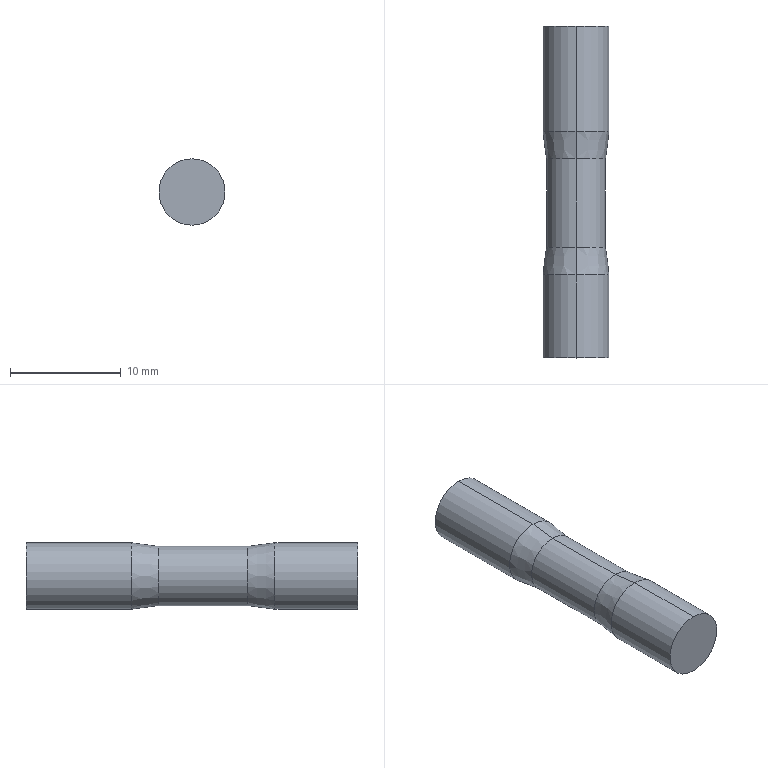Part | SolidWorks | features Revolution 1 | 1 solid | 12 faces | box 6 x 30 x 6 mm | volume 787.114 mm3 | cylinder 6 | cone 4 | plane 2 | commonest cylinder face diameters 6 x4 5.35 x2
STEP:
#1=CARTESIAN_POINT('',(0.,-22.5,-3.));
#2=VERTEX_POINT('',#1);
#3=CARTESIAN_POINT('',(0.,-22.5,3.));
#4=VERTEX_POINT('',#3);
#5=CARTESIAN_POINT('',(0.,-22.5,0.));
#6=DIRECTION('',(0.,-1.,0.));
#7=DIRECTION('',(0.,0.,-1.));
#8=AXIS2_PLACEMENT_3D('',#5,#6,#7);
#9=CIRCLE('',#8,3.);
#10=EDGE_CURVE('',#2,#4,#9,.T.);
#11=ORIENTED_EDGE('',*,*,#10,.T.);
#12=CARTESIAN_POINT('',(0.,-30.,3.));
#13=VERTEX_POINT('',#12);
#14=CARTESIAN_POINT('',(0.,-30.,3.));
#15=DIRECTION('',(0.,-1.,0.));
#16=VECTOR('',#15,1000.);
#17=LINE('',#14,#16);
#18=EDGE_CURVE('',#4,#13,#17,.T.);
#19=ORIENTED_EDGE('',*,*,#18,.T.);
#20=CARTESIAN_POINT('',(0.,-30.,-3.));
#21=VERTEX_POINT('',#20);
#22=CARTESIAN_POINT('',(0.,-30.,0.));
#23=DIRECTION('',(0.,-1.,0.));
#24=DIRECTION('',(0.,0.,-1.));
#25=AXIS2_PLACEMENT_3D('',#22,#23,#24);
#26=CIRCLE('',#25,3.);
#27=EDGE_CURVE('',#21,#13,#26,.T.);
#28=ORIENTED_EDGE('',*,*,#27,.F.);
#29=CARTESIAN_POINT('',(0.,-30.,-3.));
#30=DIRECTION('',(0.,-1.,0.));
#31=VECTOR('',#30,1000.);
#32=LINE('',#29,#31);
#33=EDGE_CURVE('',#2,#21,#32,.T.);
#34=ORIENTED_EDGE('',*,*,#33,.F.);
#35=EDGE_LOOP('',(#11,#19,#28,#34));
#36=FACE_OUTER_BOUND('',#35,.T.);
#37=CARTESIAN_POINT('',(0.,-30.,0.));
#38=DIRECTION('',(0.,-1.,0.));
#39=DIRECTION('',(0.,0.,-1.));
#40=AXIS2_PLACEMENT_3D('',#37,#38,#39);
#41=CYLINDRICAL_SURFACE('',#40,3.);
#42=ADVANCED_FACE('',(#36),#41,.T.);
#43=CARTESIAN_POINT('',(0.,-20.,-2.675));
#44=VERTEX_POINT('',#43);
#45=CARTESIAN_POINT('',(0.,-20.,2.675));
#46=VERTEX_POINT('',#45);
#47=CARTESIAN_POINT('',(0.,-20.,0.));
#48=DIRECTION('',(0.,-1.,0.));
#49=DIRECTION('',(0.,0.,-1.));
#50=AXIS2_PLACEMENT_3D('',#47,#48,#49);
#51=CIRCLE('',#50,2.675);
#52=EDGE_CURVE('',#44,#46,#51,.T.);
#53=ORIENTED_EDGE('',*,*,#52,.T.);
#54=CARTESIAN_POINT('',(0.,-20.,2.675));
#55=DIRECTION('',(0.,-0.9917,0.1289));
#56=VECTOR('',#55,1000.);
#57=LINE('',#54,#56);
#58=EDGE_CURVE('',#46,#4,#57,.T.);
#59=ORIENTED_EDGE('',*,*,#58,.T.);
#60=ORIENTED_EDGE('',*,*,#10,.F.);
#61=CARTESIAN_POINT('',(0.,-20.,-2.675));
#62=DIRECTION('',(0.,-0.9917,-0.1289));
#63=VECTOR('',#62,1000.);
#64=LINE('',#61,#63);
#65=EDGE_CURVE('',#44,#2,#64,.T.);
#66=ORIENTED_EDGE('',*,*,#65,.F.);
#67=EDGE_LOOP('',(#53,#59,#60,#66));
#68=FACE_OUTER_BOUND('',#67,.T.);
#69=CARTESIAN_POINT('',(0.,-20.,0.));
#70=DIRECTION('',(0.,-1.,0.));
#71=DIRECTION('',(0.,0.,-1.));
#72=AXIS2_PLACEMENT_3D('',#69,#70,#71);
#73=CONICAL_SURFACE('',#72,2.675,0.1293);
#74=ADVANCED_FACE('',(#68),#73,.T.);
#75=CARTESIAN_POINT('',(0.,-12.,-2.675));
#76=VERTEX_POINT('',#75);
#77=CARTESIAN_POINT('',(0.,-12.,2.675));
#78=VERTEX_POINT('',#77);
#79=CARTESIAN_POINT('',(0.,-12.,0.));
#80=DIRECTION('',(0.,-1.,0.));
#81=DIRECTION('',(0.,0.,-1.));
#82=AXIS2_PLACEMENT_3D('',#79,#80,#81);
#83=CIRCLE('',#82,2.675);
#84=EDGE_CURVE('',#76,#78,#83,.T.);
#85=ORIENTED_EDGE('',*,*,#84,.T.);
#86=CARTESIAN_POINT('',(0.,-30.,2.675));
#87=DIRECTION('',(0.,-1.,0.));
#88=VECTOR('',#87,1000.);
#89=LINE('',#86,#88);
#90=EDGE_CURVE('',#78,#46,#89,.T.);
#91=ORIENTED_EDGE('',*,*,#90,.T.);
#92=ORIENTED_EDGE('',*,*,#52,.F.);
#93=CARTESIAN_POINT('',(0.,-30.,-2.675));
#94=DIRECTION('',(0.,-1.,0.));
#95=VECTOR('',#94,1000.);
#96=LINE('',#93,#95);
#97=EDGE_CURVE('',#76,#44,#96,.T.);
#98=ORIENTED_EDGE('',*,*,#97,.F.);
#99=EDGE_LOOP('',(#85,#91,#92,#98));
#100=FACE_OUTER_BOUND('',#99,.T.);
#101=CARTESIAN_POINT('',(0.,-30.,0.));
#102=DIRECTION('',(0.,-1.,0.));
#103=DIRECTION('',(0.,0.,-1.));
#104=AXIS2_PLACEMENT_3D('',#101,#102,#103);
#105=CYLINDRICAL_SURFACE('',#104,2.675);
#106=ADVANCED_FACE('',(#100),#105,.T.);
#107=ORIENTED_EDGE('',*,*,#84,.F.);
#108=CARTESIAN_POINT('',(0.,-9.5,-3.));
#109=VERTEX_POINT('',#108);
#110=CARTESIAN_POINT('',(0.,-9.5,-3.));
#111=DIRECTION('',(0.,0.9917,-0.1289));
#112=VECTOR('',#111,1000.);
#113=LINE('',#110,#112);
#114=EDGE_CURVE('',#76,#109,#113,.T.);
#115=ORIENTED_EDGE('',*,*,#114,.T.);
#116=CARTESIAN_POINT('',(0.,-9.5,3.));
#117=VERTEX_POINT('',#116);
#118=CARTESIAN_POINT('',(0.,-9.5,0.));
#119=DIRECTION('',(0.,-1.,0.));
#120=DIRECTION('',(0.,0.,-1.));
#121=AXIS2_PLACEMENT_3D('',#118,#119,#120);
#122=CIRCLE('',#121,3.);
#123=EDGE_CURVE('',#109,#117,#122,.T.);
#124=ORIENTED_EDGE('',*,*,#123,.T.);
#125=CARTESIAN_POINT('',(0.,-9.5,3.));
#126=DIRECTION('',(0.,0.9917,0.1289));
#127=VECTOR('',#126,1000.);
#128=LINE('',#125,#127);
#129=EDGE_CURVE('',#78,#117,#128,.T.);
#130=ORIENTED_EDGE('',*,*,#129,.F.);
#131=EDGE_LOOP('',(#107,#115,#124,#130));
#132=FACE_OUTER_BOUND('',#131,.T.);
#133=CARTESIAN_POINT('',(0.,-9.5,0.));
#134=DIRECTION('',(0.,1.,0.));
#135=DIRECTION('',(0.,0.,1.));
#136=AXIS2_PLACEMENT_3D('',#133,#134,#135);
#137=CONICAL_SURFACE('',#136,3.,0.1293);
#138=ADVANCED_FACE('',(#132),#137,.T.);
#139=CARTESIAN_POINT('',(0.,0.,-3.));
#140=VERTEX_POINT('',#139);
#141=CARTESIAN_POINT('',(0.,0.,3.));
#142=VERTEX_POINT('',#141);
#143=CARTESIAN_POINT('',(0.,0.,0.));
#144=DIRECTION('',(0.,-1.,0.));
#145=DIRECTION('',(0.,0.,-1.));
#146=AXIS2_PLACEMENT_3D('',#143,#144,#145);
#147=CIRCLE('',#146,3.);
#148=EDGE_CURVE('',#140,#142,#147,.T.);
#149=ORIENTED_EDGE('',*,*,#148,.T.);
#150=CARTESIAN_POINT('',(0.,-30.,3.));
#151=DIRECTION('',(0.,-1.,0.));
#152=VECTOR('',#151,1000.);
#153=LINE('',#150,#152);
#154=EDGE_CURVE('',#142,#117,#153,.T.);
#155=ORIENTED_EDGE('',*,*,#154,.T.);
#156=ORIENTED_EDGE('',*,*,#123,.F.);
#157=CARTESIAN_POINT('',(0.,-30.,-3.));
#158=DIRECTION('',(0.,-1.,0.));
#159=VECTOR('',#158,1000.);
#160=LINE('',#157,#159);
#161=EDGE_CURVE('',#140,#109,#160,.T.);
#162=ORIENTED_EDGE('',*,*,#161,.F.);
#163=EDGE_LOOP('',(#149,#155,#156,#162));
#164=FACE_OUTER_BOUND('',#163,.T.);
#165=CARTESIAN_POINT('',(0.,-30.,0.));
#166=DIRECTION('',(0.,-1.,0.));
#167=DIRECTION('',(0.,0.,-1.));
#168=AXIS2_PLACEMENT_3D('',#165,#166,#167);
#169=CYLINDRICAL_SURFACE('',#168,3.);
#170=ADVANCED_FACE('',(#164),#169,.T.);
#171=ORIENTED_EDGE('',*,*,#148,.F.);
#172=CARTESIAN_POINT('',(0.,0.,0.));
#173=DIRECTION('',(0.,-1.,0.));
#174=DIRECTION('',(0.,0.,-1.));
#175=AXIS2_PLACEMENT_3D('',#172,#173,#174);
#176=CIRCLE('',#175,3.);
#177=EDGE_CURVE('',#142,#140,#176,.T.);
#178=ORIENTED_EDGE('',*,*,#177,.F.);
#179=EDGE_LOOP('',(#171,#178));
#180=FACE_OUTER_BOUND('',#179,.T.);
#181=CARTESIAN_POINT('',(0.,0.,0.));
#182=DIRECTION('',(0.,-1.,0.));
#183=DIRECTION('',(0.,0.,-1.));
#184=AXIS2_PLACEMENT_3D('',#181,#182,#183);
#185=PLANE('',#184);
#186=ADVANCED_FACE('',(#180),#185,.F.);
#187=ORIENTED_EDGE('',*,*,#154,.F.);
#188=ORIENTED_EDGE('',*,*,#177,.T.);
#189=ORIENTED_EDGE('',*,*,#161,.T.);
#190=CARTESIAN_POINT('',(0.,-9.5,0.));
#191=DIRECTION('',(0.,-1.,0.));
#192=DIRECTION('',(0.,0.,-1.));
#193=AXIS2_PLACEMENT_3D('',#190,#191,#192);
#194=CIRCLE('',#193,3.);
#195=EDGE_CURVE('',#117,#109,#194,.T.);
#196=ORIENTED_EDGE('',*,*,#195,.F.);
#197=EDGE_LOOP('',(#187,#188,#189,#196));
#198=FACE_OUTER_BOUND('',#197,.T.);
#199=CARTESIAN_POINT('',(0.,-30.,0.));
#200=DIRECTION('',(0.,-1.,0.));
#201=DIRECTION('',(0.,0.,-1.));
#202=AXIS2_PLACEMENT_3D('',#199,#200,#201);
#203=CYLINDRICAL_SURFACE('',#202,3.);
#204=ADVANCED_FACE('',(#198),#203,.T.);
#205=ORIENTED_EDGE('',*,*,#114,.F.);
#206=CARTESIAN_POINT('',(0.,-12.,0.));
#207=DIRECTION('',(0.,-1.,0.));
#208=DIRECTION('',(0.,0.,-1.));
#209=AXIS2_PLACEMENT_3D('',#206,#207,#208);
#210=CIRCLE('',#209,2.675);
#211=EDGE_CURVE('',#78,#76,#210,.T.);
#212=ORIENTED_EDGE('',*,*,#211,.F.);
#213=ORIENTED_EDGE('',*,*,#129,.T.);
#214=ORIENTED_EDGE('',*,*,#195,.T.);
#215=EDGE_LOOP('',(#205,#212,#213,#214));
#216=FACE_OUTER_BOUND('',#215,.T.);
#217=CARTESIAN_POINT('',(0.,-9.5,0.));
#218=DIRECTION('',(0.,1.,0.));
#219=DIRECTION('',(0.,0.,1.));
#220=AXIS2_PLACEMENT_3D('',#217,#218,#219);
#221=CONICAL_SURFACE('',#220,3.,0.1293);
#222=ADVANCED_FACE('',(#216),#221,.T.);
#223=ORIENTED_EDGE('',*,*,#90,.F.);
#224=ORIENTED_EDGE('',*,*,#211,.T.);
#225=ORIENTED_EDGE('',*,*,#97,.T.);
#226=CARTESIAN_POINT('',(0.,-20.,0.));
#227=DIRECTION('',(0.,-1.,0.));
#228=DIRECTION('',(0.,0.,-1.));
#229=AXIS2_PLACEMENT_3D('',#226,#227,#228);
#230=CIRCLE('',#229,2.675);
#231=EDGE_CURVE('',#46,#44,#230,.T.);
#232=ORIENTED_EDGE('',*,*,#231,.F.);
#233=EDGE_LOOP('',(#223,#224,#225,#232));
#234=FACE_OUTER_BOUND('',#233,.T.);
#235=CARTESIAN_POINT('',(0.,-30.,0.));
#236=DIRECTION('',(0.,-1.,0.));
#237=DIRECTION('',(0.,0.,-1.));
#238=AXIS2_PLACEMENT_3D('',#235,#236,#237);
#239=CYLINDRICAL_SURFACE('',#238,2.675);
#240=ADVANCED_FACE('',(#234),#239,.T.);
#241=ORIENTED_EDGE('',*,*,#58,.F.);
#242=ORIENTED_EDGE('',*,*,#231,.T.);
#243=ORIENTED_EDGE('',*,*,#65,.T.);
#244=CARTESIAN_POINT('',(0.,-22.5,0.));
#245=DIRECTION('',(0.,-1.,0.));
#246=DIRECTION('',(0.,0.,-1.));
#247=AXIS2_PLACEMENT_3D('',#244,#245,#246);
#248=CIRCLE('',#247,3.);
#249=EDGE_CURVE('',#4,#2,#248,.T.);
#250=ORIENTED_EDGE('',*,*,#249,.F.);
#251=EDGE_LOOP('',(#241,#242,#243,#250));
#252=FACE_OUTER_BOUND('',#251,.T.);
#253=CARTESIAN_POINT('',(0.,-20.,0.));
#254=DIRECTION('',(0.,-1.,0.));
#255=DIRECTION('',(0.,0.,-1.));
#256=AXIS2_PLACEMENT_3D('',#253,#254,#255);
#257=CONICAL_SURFACE('',#256,2.675,0.1293);
#258=ADVANCED_FACE('',(#252),#257,.T.);
#259=ORIENTED_EDGE('',*,*,#18,.F.);
#260=ORIENTED_EDGE('',*,*,#249,.T.);
#261=ORIENTED_EDGE('',*,*,#33,.T.);
#262=CARTESIAN_POINT('',(0.,-30.,0.));
#263=DIRECTION('',(0.,-1.,0.));
#264=DIRECTION('',(0.,0.,-1.));
#265=AXIS2_PLACEMENT_3D('',#262,#263,#264);
#266=CIRCLE('',#265,3.);
#267=EDGE_CURVE('',#13,#21,#266,.T.);
#268=ORIENTED_EDGE('',*,*,#267,.F.);
#269=EDGE_LOOP('',(#259,#260,#261,#268));
#270=FACE_OUTER_BOUND('',#269,.T.);
#271=CARTESIAN_POINT('',(0.,-30.,0.));
#272=DIRECTION('',(0.,-1.,0.));
#273=DIRECTION('',(0.,0.,-1.));
#274=AXIS2_PLACEMENT_3D('',#271,#272,#273);
#275=CYLINDRICAL_SURFACE('',#274,3.);
#276=ADVANCED_FACE('',(#270),#275,.T.);
#277=ORIENTED_EDGE('',*,*,#27,.T.);
#278=ORIENTED_EDGE('',*,*,#267,.T.);
#279=EDGE_LOOP('',(#277,#278));
#280=FACE_OUTER_BOUND('',#279,.T.);
#281=CARTESIAN_POINT('',(-3.,-30.,0.));
#282=DIRECTION('',(0.,1.,0.));
#283=DIRECTION('',(0.,0.,1.));
#284=AXIS2_PLACEMENT_3D('',#281,#282,#283);
#285=PLANE('',#284);
#286=ADVANCED_FACE('',(#280),#285,.F.);
#287=CLOSED_SHELL('',(#42,#74,#106,#138,#170,#186,#204,#222,#240,#258,#276,#286));
#288=MANIFOLD_SOLID_BREP('',#287);
#289=CARTESIAN_POINT('',(0.,0.,0.));
#290=DIRECTION('',(0.,0.,1.));
#291=DIRECTION('',(1.,0.,0.));
#292=AXIS2_PLACEMENT_3D('',#289,#290,#291);
#293=(LENGTH_UNIT()NAMED_UNIT(*)SI_UNIT(.MILLI.,.METRE.));
#294=UNCERTAINTY_MEASURE_WITH_UNIT(LENGTH_MEASURE(0.00001),#293,'','');
#295=(NAMED_UNIT(*)PLANE_ANGLE_UNIT()SI_UNIT($,.RADIAN.));
#296=(NAMED_UNIT(*)SI_UNIT($,.STERADIAN.)SOLID_ANGLE_UNIT());
#297=(GEOMETRIC_REPRESENTATION_CONTEXT(3)GLOBAL_UNCERTAINTY_ASSIGNED_CONTEXT((#294))GLOBAL_UNIT_ASSIGNED_CONTEXT((#293,#295,#296))REPRESENTATION_CONTEXT('',''));
#298=ADVANCED_BREP_SHAPE_REPRESENTATION('',(#288,#292),#297);